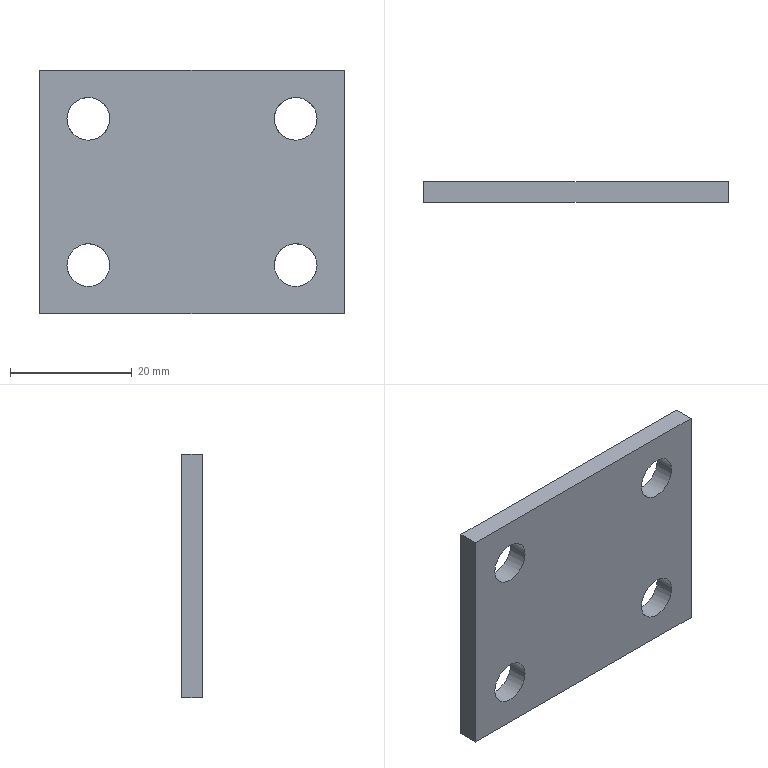Part | STEP file | Positioning_id2146_x_t | 1 solid | 14 faces | box 50 x 3.35 x 40 mm | volume 6184 mm3 | cylinder 8 | plane 6 | commonest cylinder face diameters 7 x8
STEP:
#1=CARTESIAN_POINT('',(0.,0.,0.));
#2=DIRECTION('',(0.,0.,1.));
#3=DIRECTION('',(1.,0.,0.));
#4=AXIS2_PLACEMENT_3D('',#1,#2,#3);
#5=CARTESIAN_POINT('',(-816.502,-53.35,344.5));
#6=VERTEX_POINT('',#5);
#7=CARTESIAN_POINT('',(-823.502,-53.35,344.5));
#8=VERTEX_POINT('',#7);
#9=CARTESIAN_POINT('',(-820.002,-53.35,344.5));
#10=DIRECTION('',(0.,-1.,0.));
#11=DIRECTION('',(1.,0.,0.));
#12=AXIS2_PLACEMENT_3D('',#9,#10,#11);
#13=CIRCLE('',#12,3.5);
#14=CARTESIAN_POINT('',(-773.002,-53.35,376.5));
#15=DIRECTION('',(0.,1.,0.));
#16=DIRECTION('',(-1.,0.,0.));
#17=AXIS2_PLACEMENT_3D('',#14,#15,#16);
#18=PLANE('',#17);
#19=CARTESIAN_POINT('',(43.5,-32.));
#20=CARTESIAN_POINT('',(43.5,-25.938));
#21=CARTESIAN_POINT('',(48.75,-28.969));
#22=CARTESIAN_POINT('',(54.,-32.));
#23=CARTESIAN_POINT('',(48.75,-35.031));
#24=CARTESIAN_POINT('',(43.5,-38.062));
#25=CARTESIAN_POINT('',(43.5,-32.));
#26=(BOUNDED_CURVE()B_SPLINE_CURVE(2,(#19,#20,#21,#22,#23,#24,#25),.UNSPECIFIED.,.T.,.F.)B_SPLINE_CURVE_WITH_KNOTS((1,2,2,2,2,1),(-2.094,0.,2.094,4.189,6.283,8.378),.UNSPECIFIED.)CURVE()GEOMETRIC_REPRESENTATION_ITEM()RATIONAL_B_SPLINE_CURVE((1.,0.5,1.,0.5,1.,0.5,1.))REPRESENTATION_ITEM(''));
#27=(GEOMETRIC_REPRESENTATION_CONTEXT(2)PARAMETRIC_REPRESENTATION_CONTEXT()REPRESENTATION_CONTEXT('',''));
#28=DEFINITIONAL_REPRESENTATION('',(#26),#27);
#29=PCURVE('',#18,#28);
#30=CARTESIAN_POINT('',(-820.002,-66.,344.5));
#31=DIRECTION('',(0.,-1.,0.));
#32=DIRECTION('',(-1.,0.,0.));
#33=AXIS2_PLACEMENT_3D('',#30,#31,#32);
#34=CYLINDRICAL_SURFACE('',#33,3.5);
#35=CARTESIAN_POINT('',(3.142,-12.65));
#36=DIRECTION('',(1.,0.));
#37=VECTOR('',#36,1.);
#38=LINE('',#35,#37);
#39=(GEOMETRIC_REPRESENTATION_CONTEXT(2)PARAMETRIC_REPRESENTATION_CONTEXT()REPRESENTATION_CONTEXT('',''));
#40=DEFINITIONAL_REPRESENTATION('',(#38),#39);
#41=PCURVE('',#34,#40);
#42=SURFACE_CURVE('',#13,(#29,#41),.PCURVE_S1.);
#43=EDGE_CURVE('',#6,#8,#42,.T.);
#44=ORIENTED_EDGE('',*,*,#43,.F.);
#45=CARTESIAN_POINT('',(-820.002,-53.35,341.));
#46=VERTEX_POINT('',#45);
#47=CARTESIAN_POINT('',(-820.002,-53.35,344.5));
#48=DIRECTION('',(0.,-1.,0.));
#49=DIRECTION('',(0.,0.,-1.));
#50=AXIS2_PLACEMENT_3D('',#47,#48,#49);
#51=CIRCLE('',#50,3.5);
#52=CARTESIAN_POINT('',(47.,-35.5));
#53=CARTESIAN_POINT('',(40.938,-35.5));
#54=CARTESIAN_POINT('',(43.969,-30.25));
#55=CARTESIAN_POINT('',(47.,-25.));
#56=CARTESIAN_POINT('',(50.031,-30.25));
#57=CARTESIAN_POINT('',(53.062,-35.5));
#58=CARTESIAN_POINT('',(47.,-35.5));
#59=(BOUNDED_CURVE()B_SPLINE_CURVE(2,(#52,#53,#54,#55,#56,#57,#58),.UNSPECIFIED.,.T.,.F.)B_SPLINE_CURVE_WITH_KNOTS((1,2,2,2,2,1),(-2.094,0.,2.094,4.189,6.283,8.378),.UNSPECIFIED.)CURVE()GEOMETRIC_REPRESENTATION_ITEM()RATIONAL_B_SPLINE_CURVE((1.,0.5,1.,0.5,1.,0.5,1.))REPRESENTATION_ITEM(''));
#60=(GEOMETRIC_REPRESENTATION_CONTEXT(2)PARAMETRIC_REPRESENTATION_CONTEXT()REPRESENTATION_CONTEXT('',''));
#61=DEFINITIONAL_REPRESENTATION('',(#59),#60);
#62=PCURVE('',#18,#61);
#63=CARTESIAN_POINT('',(-820.002,-66.,344.5));
#64=DIRECTION('',(0.,-1.,0.));
#65=DIRECTION('',(-1.,0.,0.));
#66=AXIS2_PLACEMENT_3D('',#63,#64,#65);
#67=CYLINDRICAL_SURFACE('',#66,3.5);
#68=CARTESIAN_POINT('',(1.571,-12.65));
#69=DIRECTION('',(1.,0.));
#70=VECTOR('',#69,1.);
#71=LINE('',#68,#70);
#72=(GEOMETRIC_REPRESENTATION_CONTEXT(2)PARAMETRIC_REPRESENTATION_CONTEXT()REPRESENTATION_CONTEXT('',''));
#73=DEFINITIONAL_REPRESENTATION('',(#71),#72);
#74=PCURVE('',#67,#73);
#75=SURFACE_CURVE('',#51,(#62,#74),.PCURVE_S1.);
#76=EDGE_CURVE('',#46,#6,#75,.T.);
#77=ORIENTED_EDGE('',*,*,#76,.F.);
#78=CARTESIAN_POINT('',(-820.002,-53.35,344.5));
#79=DIRECTION('',(0.,-1.,0.));
#80=DIRECTION('',(-1.,0.,0.));
#81=AXIS2_PLACEMENT_3D('',#78,#79,#80);
#82=CIRCLE('',#81,3.5);
#83=CARTESIAN_POINT('',(50.5,-32.));
#84=CARTESIAN_POINT('',(50.5,-38.062));
#85=CARTESIAN_POINT('',(45.25,-35.031));
#86=CARTESIAN_POINT('',(40.,-32.));
#87=CARTESIAN_POINT('',(45.25,-28.969));
#88=CARTESIAN_POINT('',(50.5,-25.938));
#89=CARTESIAN_POINT('',(50.5,-32.));
#90=(BOUNDED_CURVE()B_SPLINE_CURVE(2,(#83,#84,#85,#86,#87,#88,#89),.UNSPECIFIED.,.T.,.F.)B_SPLINE_CURVE_WITH_KNOTS((1,2,2,2,2,1),(-2.094,0.,2.094,4.189,6.283,8.378),.UNSPECIFIED.)CURVE()GEOMETRIC_REPRESENTATION_ITEM()RATIONAL_B_SPLINE_CURVE((1.,0.5,1.,0.5,1.,0.5,1.))REPRESENTATION_ITEM(''));
#91=(GEOMETRIC_REPRESENTATION_CONTEXT(2)PARAMETRIC_REPRESENTATION_CONTEXT()REPRESENTATION_CONTEXT('',''));
#92=DEFINITIONAL_REPRESENTATION('',(#90),#91);
#93=PCURVE('',#18,#92);
#94=CARTESIAN_POINT('',(0.,-12.65));
#95=DIRECTION('',(1.,0.));
#96=VECTOR('',#95,1.);
#97=LINE('',#94,#96);
#98=(GEOMETRIC_REPRESENTATION_CONTEXT(2)PARAMETRIC_REPRESENTATION_CONTEXT()REPRESENTATION_CONTEXT('',''));
#99=DEFINITIONAL_REPRESENTATION('',(#97),#98);
#100=PCURVE('',#67,#99);
#101=SURFACE_CURVE('',#82,(#93,#100),.PCURVE_S1.);
#102=EDGE_CURVE('',#8,#46,#101,.T.);
#103=ORIENTED_EDGE('',*,*,#102,.F.);
#104=EDGE_LOOP('',(#44,#77,#103));
#105=FACE_BOUND('',#104,.T.);
#106=CARTESIAN_POINT('',(-782.502,-53.35,368.5));
#107=VERTEX_POINT('',#106);
#108=CARTESIAN_POINT('',(-789.502,-53.35,368.5));
#109=VERTEX_POINT('',#108);
#110=CARTESIAN_POINT('',(-786.002,-53.35,368.5));
#111=DIRECTION('',(0.,-1.,0.));
#112=DIRECTION('',(1.,0.,0.));
#113=AXIS2_PLACEMENT_3D('',#110,#111,#112);
#114=CIRCLE('',#113,3.5);
#115=CARTESIAN_POINT('',(9.5,-8.));
#116=CARTESIAN_POINT('',(9.5,-1.938));
#117=CARTESIAN_POINT('',(14.75,-4.969));
#118=CARTESIAN_POINT('',(20.,-8.));
#119=CARTESIAN_POINT('',(14.75,-11.031));
#120=CARTESIAN_POINT('',(9.5,-14.062));
#121=CARTESIAN_POINT('',(9.5,-8.));
#122=(BOUNDED_CURVE()B_SPLINE_CURVE(2,(#115,#116,#117,#118,#119,#120,#121),.UNSPECIFIED.,.T.,.F.)B_SPLINE_CURVE_WITH_KNOTS((1,2,2,2,2,1),(-2.094,0.,2.094,4.189,6.283,8.378),.UNSPECIFIED.)CURVE()GEOMETRIC_REPRESENTATION_ITEM()RATIONAL_B_SPLINE_CURVE((1.,0.5,1.,0.5,1.,0.5,1.))REPRESENTATION_ITEM(''));
#123=(GEOMETRIC_REPRESENTATION_CONTEXT(2)PARAMETRIC_REPRESENTATION_CONTEXT()REPRESENTATION_CONTEXT('',''));
#124=DEFINITIONAL_REPRESENTATION('',(#122),#123);
#125=PCURVE('',#18,#124);
#126=CARTESIAN_POINT('',(-786.002,-66.,368.5));
#127=DIRECTION('',(0.,-1.,0.));
#128=DIRECTION('',(-1.,0.,0.));
#129=AXIS2_PLACEMENT_3D('',#126,#127,#128);
#130=CYLINDRICAL_SURFACE('',#129,3.5);
#131=CARTESIAN_POINT('',(3.142,-12.65));
#132=DIRECTION('',(1.,0.));
#133=VECTOR('',#132,1.);
#134=LINE('',#131,#133);
#135=(GEOMETRIC_REPRESENTATION_CONTEXT(2)PARAMETRIC_REPRESENTATION_CONTEXT()REPRESENTATION_CONTEXT('',''));
#136=DEFINITIONAL_REPRESENTATION('',(#134),#135);
#137=PCURVE('',#130,#136);
#138=SURFACE_CURVE('',#114,(#125,#137),.PCURVE_S1.);
#139=EDGE_CURVE('',#107,#109,#138,.T.);
#140=ORIENTED_EDGE('',*,*,#139,.F.);
#141=CARTESIAN_POINT('',(-786.002,-53.35,365.));
#142=VERTEX_POINT('',#141);
#143=CARTESIAN_POINT('',(-786.002,-53.35,368.5));
#144=DIRECTION('',(0.,-1.,0.));
#145=DIRECTION('',(0.,0.,-1.));
#146=AXIS2_PLACEMENT_3D('',#143,#144,#145);
#147=CIRCLE('',#146,3.5);
#148=CARTESIAN_POINT('',(13.,-11.5));
#149=CARTESIAN_POINT('',(6.938,-11.5));
#150=CARTESIAN_POINT('',(9.969,-6.25));
#151=CARTESIAN_POINT('',(13.,-1.));
#152=CARTESIAN_POINT('',(16.031,-6.25));
#153=CARTESIAN_POINT('',(19.062,-11.5));
#154=CARTESIAN_POINT('',(13.,-11.5));
#155=(BOUNDED_CURVE()B_SPLINE_CURVE(2,(#148,#149,#150,#151,#152,#153,#154),.UNSPECIFIED.,.T.,.F.)B_SPLINE_CURVE_WITH_KNOTS((1,2,2,2,2,1),(-2.094,0.,2.094,4.189,6.283,8.378),.UNSPECIFIED.)CURVE()GEOMETRIC_REPRESENTATION_ITEM()RATIONAL_B_SPLINE_CURVE((1.,0.5,1.,0.5,1.,0.5,1.))REPRESENTATION_ITEM(''));
#156=(GEOMETRIC_REPRESENTATION_CONTEXT(2)PARAMETRIC_REPRESENTATION_CONTEXT()REPRESENTATION_CONTEXT('',''));
#157=DEFINITIONAL_REPRESENTATION('',(#155),#156);
#158=PCURVE('',#18,#157);
#159=CARTESIAN_POINT('',(-786.002,-66.,368.5));
#160=DIRECTION('',(0.,-1.,0.));
#161=DIRECTION('',(-1.,0.,0.));
#162=AXIS2_PLACEMENT_3D('',#159,#160,#161);
#163=CYLINDRICAL_SURFACE('',#162,3.5);
#164=CARTESIAN_POINT('',(1.571,-12.65));
#165=DIRECTION('',(1.,0.));
#166=VECTOR('',#165,1.);
#167=LINE('',#164,#166);
#168=(GEOMETRIC_REPRESENTATION_CONTEXT(2)PARAMETRIC_REPRESENTATION_CONTEXT()REPRESENTATION_CONTEXT('',''));
#169=DEFINITIONAL_REPRESENTATION('',(#167),#168);
#170=PCURVE('',#163,#169);
#171=SURFACE_CURVE('',#147,(#158,#170),.PCURVE_S1.);
#172=EDGE_CURVE('',#142,#107,#171,.T.);
#173=ORIENTED_EDGE('',*,*,#172,.F.);
#174=CARTESIAN_POINT('',(-786.002,-53.35,368.5));
#175=DIRECTION('',(0.,-1.,0.));
#176=DIRECTION('',(-1.,0.,0.));
#177=AXIS2_PLACEMENT_3D('',#174,#175,#176);
#178=CIRCLE('',#177,3.5);
#179=CARTESIAN_POINT('',(16.5,-8.));
#180=CARTESIAN_POINT('',(16.5,-14.062));
#181=CARTESIAN_POINT('',(11.25,-11.031));
#182=CARTESIAN_POINT('',(6.,-8.));
#183=CARTESIAN_POINT('',(11.25,-4.969));
#184=CARTESIAN_POINT('',(16.5,-1.938));
#185=CARTESIAN_POINT('',(16.5,-8.));
#186=(BOUNDED_CURVE()B_SPLINE_CURVE(2,(#179,#180,#181,#182,#183,#184,#185),.UNSPECIFIED.,.T.,.F.)B_SPLINE_CURVE_WITH_KNOTS((1,2,2,2,2,1),(-2.094,0.,2.094,4.189,6.283,8.378),.UNSPECIFIED.)CURVE()GEOMETRIC_REPRESENTATION_ITEM()RATIONAL_B_SPLINE_CURVE((1.,0.5,1.,0.5,1.,0.5,1.))REPRESENTATION_ITEM(''));
#187=(GEOMETRIC_REPRESENTATION_CONTEXT(2)PARAMETRIC_REPRESENTATION_CONTEXT()REPRESENTATION_CONTEXT('',''));
#188=DEFINITIONAL_REPRESENTATION('',(#186),#187);
#189=PCURVE('',#18,#188);
#190=CARTESIAN_POINT('',(0.,-12.65));
#191=DIRECTION('',(1.,0.));
#192=VECTOR('',#191,1.);
#193=LINE('',#190,#192);
#194=(GEOMETRIC_REPRESENTATION_CONTEXT(2)PARAMETRIC_REPRESENTATION_CONTEXT()REPRESENTATION_CONTEXT('',''));
#195=DEFINITIONAL_REPRESENTATION('',(#193),#194);
#196=PCURVE('',#163,#195);
#197=SURFACE_CURVE('',#178,(#189,#196),.PCURVE_S1.);
#198=EDGE_CURVE('',#109,#142,#197,.T.);
#199=ORIENTED_EDGE('',*,*,#198,.F.);
#200=EDGE_LOOP('',(#140,#173,#199));
#201=FACE_BOUND('',#200,.T.);
#202=CARTESIAN_POINT('',(-782.502,-53.35,344.5));
#203=VERTEX_POINT('',#202);
#204=CARTESIAN_POINT('',(-789.502,-53.35,344.5));
#205=VERTEX_POINT('',#204);
#206=CARTESIAN_POINT('',(-786.002,-53.35,344.5));
#207=DIRECTION('',(0.,-1.,0.));
#208=DIRECTION('',(1.,0.,0.));
#209=AXIS2_PLACEMENT_3D('',#206,#207,#208);
#210=CIRCLE('',#209,3.5);
#211=CARTESIAN_POINT('',(9.5,-32.));
#212=CARTESIAN_POINT('',(9.5,-25.938));
#213=CARTESIAN_POINT('',(14.75,-28.969));
#214=CARTESIAN_POINT('',(20.,-32.));
#215=CARTESIAN_POINT('',(14.75,-35.031));
#216=CARTESIAN_POINT('',(9.5,-38.062));
#217=CARTESIAN_POINT('',(9.5,-32.));
#218=(BOUNDED_CURVE()B_SPLINE_CURVE(2,(#211,#212,#213,#214,#215,#216,#217),.UNSPECIFIED.,.T.,.F.)B_SPLINE_CURVE_WITH_KNOTS((1,2,2,2,2,1),(-2.094,0.,2.094,4.189,6.283,8.378),.UNSPECIFIED.)CURVE()GEOMETRIC_REPRESENTATION_ITEM()RATIONAL_B_SPLINE_CURVE((1.,0.5,1.,0.5,1.,0.5,1.))REPRESENTATION_ITEM(''));
#219=(GEOMETRIC_REPRESENTATION_CONTEXT(2)PARAMETRIC_REPRESENTATION_CONTEXT()REPRESENTATION_CONTEXT('',''));
#220=DEFINITIONAL_REPRESENTATION('',(#218),#219);
#221=PCURVE('',#18,#220);
#222=CARTESIAN_POINT('',(-786.002,-66.,344.5));
#223=DIRECTION('',(0.,-1.,0.));
#224=DIRECTION('',(-1.,0.,0.));
#225=AXIS2_PLACEMENT_3D('',#222,#223,#224);
#226=CYLINDRICAL_SURFACE('',#225,3.5);
#227=CARTESIAN_POINT('',(3.142,-12.65));
#228=DIRECTION('',(1.,0.));
#229=VECTOR('',#228,1.);
#230=LINE('',#227,#229);
#231=(GEOMETRIC_REPRESENTATION_CONTEXT(2)PARAMETRIC_REPRESENTATION_CONTEXT()REPRESENTATION_CONTEXT('',''));
#232=DEFINITIONAL_REPRESENTATION('',(#230),#231);
#233=PCURVE('',#226,#232);
#234=SURFACE_CURVE('',#210,(#221,#233),.PCURVE_S1.);
#235=EDGE_CURVE('',#203,#205,#234,.T.);
#236=ORIENTED_EDGE('',*,*,#235,.F.);
#237=CARTESIAN_POINT('',(-786.002,-53.35,341.));
#238=VERTEX_POINT('',#237);
#239=CARTESIAN_POINT('',(-786.002,-53.35,344.5));
#240=DIRECTION('',(0.,-1.,0.));
#241=DIRECTION('',(0.,0.,-1.));
#242=AXIS2_PLACEMENT_3D('',#239,#240,#241);
#243=CIRCLE('',#242,3.5);
#244=CARTESIAN_POINT('',(13.,-35.5));
#245=CARTESIAN_POINT('',(6.938,-35.5));
#246=CARTESIAN_POINT('',(9.969,-30.25));
#247=CARTESIAN_POINT('',(13.,-25.));
#248=CARTESIAN_POINT('',(16.031,-30.25));
#249=CARTESIAN_POINT('',(19.062,-35.5));
#250=CARTESIAN_POINT('',(13.,-35.5));
#251=(BOUNDED_CURVE()B_SPLINE_CURVE(2,(#244,#245,#246,#247,#248,#249,#250),.UNSPECIFIED.,.T.,.F.)B_SPLINE_CURVE_WITH_KNOTS((1,2,2,2,2,1),(-2.094,0.,2.094,4.189,6.283,8.378),.UNSPECIFIED.)CURVE()GEOMETRIC_REPRESENTATION_ITEM()RATIONAL_B_SPLINE_CURVE((1.,0.5,1.,0.5,1.,0.5,1.))REPRESENTATION_ITEM(''));
#252=(GEOMETRIC_REPRESENTATION_CONTEXT(2)PARAMETRIC_REPRESENTATION_CONTEXT()REPRESENTATION_CONTEXT('',''));
#253=DEFINITIONAL_REPRESENTATION('',(#251),#252);
#254=PCURVE('',#18,#253);
#255=CARTESIAN_POINT('',(-786.002,-66.,344.5));
#256=DIRECTION('',(0.,-1.,0.));
#257=DIRECTION('',(-1.,0.,0.));
#258=AXIS2_PLACEMENT_3D('',#255,#256,#257);
#259=CYLINDRICAL_SURFACE('',#258,3.5);
#260=CARTESIAN_POINT('',(1.571,-12.65));
#261=DIRECTION('',(1.,0.));
#262=VECTOR('',#261,1.);
#263=LINE('',#260,#262);
#264=(GEOMETRIC_REPRESENTATION_CONTEXT(2)PARAMETRIC_REPRESENTATION_CONTEXT()REPRESENTATION_CONTEXT('',''));
#265=DEFINITIONAL_REPRESENTATION('',(#263),#264);
#266=PCURVE('',#259,#265);
#267=SURFACE_CURVE('',#243,(#254,#266),.PCURVE_S1.);
#268=EDGE_CURVE('',#238,#203,#267,.T.);
#269=ORIENTED_EDGE('',*,*,#268,.F.);
#270=CARTESIAN_POINT('',(-786.002,-53.35,344.5));
#271=DIRECTION('',(0.,-1.,0.));
#272=DIRECTION('',(-1.,0.,0.));
#273=AXIS2_PLACEMENT_3D('',#270,#271,#272);
#274=CIRCLE('',#273,3.5);
#275=CARTESIAN_POINT('',(16.5,-32.));
#276=CARTESIAN_POINT('',(16.5,-38.062));
#277=CARTESIAN_POINT('',(11.25,-35.031));
#278=CARTESIAN_POINT('',(6.,-32.));
#279=CARTESIAN_POINT('',(11.25,-28.969));
#280=CARTESIAN_POINT('',(16.5,-25.938));
#281=CARTESIAN_POINT('',(16.5,-32.));
#282=(BOUNDED_CURVE()B_SPLINE_CURVE(2,(#275,#276,#277,#278,#279,#280,#281),.UNSPECIFIED.,.T.,.F.)B_SPLINE_CURVE_WITH_KNOTS((1,2,2,2,2,1),(-2.094,0.,2.094,4.189,6.283,8.378),.UNSPECIFIED.)CURVE()GEOMETRIC_REPRESENTATION_ITEM()RATIONAL_B_SPLINE_CURVE((1.,0.5,1.,0.5,1.,0.5,1.))REPRESENTATION_ITEM(''));
#283=(GEOMETRIC_REPRESENTATION_CONTEXT(2)PARAMETRIC_REPRESENTATION_CONTEXT()REPRESENTATION_CONTEXT('',''));
#284=DEFINITIONAL_REPRESENTATION('',(#282),#283);
#285=PCURVE('',#18,#284);
#286=CARTESIAN_POINT('',(0.,-12.65));
#287=DIRECTION('',(1.,0.));
#288=VECTOR('',#287,1.);
#289=LINE('',#286,#288);
#290=(GEOMETRIC_REPRESENTATION_CONTEXT(2)PARAMETRIC_REPRESENTATION_CONTEXT()REPRESENTATION_CONTEXT('',''));
#291=DEFINITIONAL_REPRESENTATION('',(#289),#290);
#292=PCURVE('',#259,#291);
#293=SURFACE_CURVE('',#274,(#285,#292),.PCURVE_S1.);
#294=EDGE_CURVE('',#205,#238,#293,.T.);
#295=ORIENTED_EDGE('',*,*,#294,.F.);
#296=EDGE_LOOP('',(#236,#269,#295));
#297=FACE_BOUND('',#296,.T.);
#298=CARTESIAN_POINT('',(-816.502,-53.35,368.5));
#299=VERTEX_POINT('',#298);
#300=CARTESIAN_POINT('',(-823.502,-53.35,368.5));
#301=VERTEX_POINT('',#300);
#302=CARTESIAN_POINT('',(-820.002,-53.35,368.5));
#303=DIRECTION('',(0.,-1.,0.));
#304=DIRECTION('',(1.,0.,0.));
#305=AXIS2_PLACEMENT_3D('',#302,#303,#304);
#306=CIRCLE('',#305,3.5);
#307=CARTESIAN_POINT('',(43.5,-8.));
#308=CARTESIAN_POINT('',(43.5,-1.938));
#309=CARTESIAN_POINT('',(48.75,-4.969));
#310=CARTESIAN_POINT('',(54.,-8.));
#311=CARTESIAN_POINT('',(48.75,-11.031));
#312=CARTESIAN_POINT('',(43.5,-14.062));
#313=CARTESIAN_POINT('',(43.5,-8.));
#314=(BOUNDED_CURVE()B_SPLINE_CURVE(2,(#307,#308,#309,#310,#311,#312,#313),.UNSPECIFIED.,.T.,.F.)B_SPLINE_CURVE_WITH_KNOTS((1,2,2,2,2,1),(-2.094,0.,2.094,4.189,6.283,8.378),.UNSPECIFIED.)CURVE()GEOMETRIC_REPRESENTATION_ITEM()RATIONAL_B_SPLINE_CURVE((1.,0.5,1.,0.5,1.,0.5,1.))REPRESENTATION_ITEM(''));
#315=(GEOMETRIC_REPRESENTATION_CONTEXT(2)PARAMETRIC_REPRESENTATION_CONTEXT()REPRESENTATION_CONTEXT('',''));
#316=DEFINITIONAL_REPRESENTATION('',(#314),#315);
#317=PCURVE('',#18,#316);
#318=CARTESIAN_POINT('',(-820.002,-66.,368.5));
#319=DIRECTION('',(0.,-1.,0.));
#320=DIRECTION('',(-1.,0.,0.));
#321=AXIS2_PLACEMENT_3D('',#318,#319,#320);
#322=CYLINDRICAL_SURFACE('',#321,3.5);
#323=CARTESIAN_POINT('',(3.142,-12.65));
#324=DIRECTION('',(1.,0.));
#325=VECTOR('',#324,1.);
#326=LINE('',#323,#325);
#327=(GEOMETRIC_REPRESENTATION_CONTEXT(2)PARAMETRIC_REPRESENTATION_CONTEXT()REPRESENTATION_CONTEXT('',''));
#328=DEFINITIONAL_REPRESENTATION('',(#326),#327);
#329=PCURVE('',#322,#328);
#330=SURFACE_CURVE('',#306,(#317,#329),.PCURVE_S1.);
#331=EDGE_CURVE('',#299,#301,#330,.T.);
#332=ORIENTED_EDGE('',*,*,#331,.F.);
#333=CARTESIAN_POINT('',(-820.002,-53.35,365.));
#334=VERTEX_POINT('',#333);
#335=CARTESIAN_POINT('',(-820.002,-53.35,368.5));
#336=DIRECTION('',(0.,-1.,0.));
#337=DIRECTION('',(0.,0.,-1.));
#338=AXIS2_PLACEMENT_3D('',#335,#336,#337);
#339=CIRCLE('',#338,3.5);
#340=CARTESIAN_POINT('',(47.,-11.5));
#341=CARTESIAN_POINT('',(40.938,-11.5));
#342=CARTESIAN_POINT('',(43.969,-6.25));
#343=CARTESIAN_POINT('',(47.,-1.));
#344=CARTESIAN_POINT('',(50.031,-6.25));
#345=CARTESIAN_POINT('',(53.062,-11.5));
#346=CARTESIAN_POINT('',(47.,-11.5));
#347=(BOUNDED_CURVE()B_SPLINE_CURVE(2,(#340,#341,#342,#343,#344,#345,#346),.UNSPECIFIED.,.T.,.F.)B_SPLINE_CURVE_WITH_KNOTS((1,2,2,2,2,1),(-2.094,0.,2.094,4.189,6.283,8.378),.UNSPECIFIED.)CURVE()GEOMETRIC_REPRESENTATION_ITEM()RATIONAL_B_SPLINE_CURVE((1.,0.5,1.,0.5,1.,0.5,1.))REPRESENTATION_ITEM(''));
#348=(GEOMETRIC_REPRESENTATION_CONTEXT(2)PARAMETRIC_REPRESENTATION_CONTEXT()REPRESENTATION_CONTEXT('',''));
#349=DEFINITIONAL_REPRESENTATION('',(#347),#348);
#350=PCURVE('',#18,#349);
#351=CARTESIAN_POINT('',(-820.002,-66.,368.5));
#352=DIRECTION('',(0.,-1.,0.));
#353=DIRECTION('',(-1.,0.,0.));
#354=AXIS2_PLACEMENT_3D('',#351,#352,#353);
#355=CYLINDRICAL_SURFACE('',#354,3.5);
#356=CARTESIAN_POINT('',(1.571,-12.65));
#357=DIRECTION('',(1.,0.));
#358=VECTOR('',#357,1.);
#359=LINE('',#356,#358);
#360=(GEOMETRIC_REPRESENTATION_CONTEXT(2)PARAMETRIC_REPRESENTATION_CONTEXT()REPRESENTATION_CONTEXT('',''));
#361=DEFINITIONAL_REPRESENTATION('',(#359),#360);
#362=PCURVE('',#355,#361);
#363=SURFACE_CURVE('',#339,(#350,#362),.PCURVE_S1.);
#364=EDGE_CURVE('',#334,#299,#363,.T.);
#365=ORIENTED_EDGE('',*,*,#364,.F.);
#366=CARTESIAN_POINT('',(-820.002,-53.35,368.5));
#367=DIRECTION('',(0.,-1.,0.));
#368=DIRECTION('',(-1.,0.,0.));
#369=AXIS2_PLACEMENT_3D('',#366,#367,#368);
#370=CIRCLE('',#369,3.5);
#371=CARTESIAN_POINT('',(50.5,-8.));
#372=CARTESIAN_POINT('',(50.5,-14.062));
#373=CARTESIAN_POINT('',(45.25,-11.031));
#374=CARTESIAN_POINT('',(40.,-8.));
#375=CARTESIAN_POINT('',(45.25,-4.969));
#376=CARTESIAN_POINT('',(50.5,-1.938));
#377=CARTESIAN_POINT('',(50.5,-8.));
#378=(BOUNDED_CURVE()B_SPLINE_CURVE(2,(#371,#372,#373,#374,#375,#376,#377),.UNSPECIFIED.,.T.,.F.)B_SPLINE_CURVE_WITH_KNOTS((1,2,2,2,2,1),(-2.094,0.,2.094,4.189,6.283,8.378),.UNSPECIFIED.)CURVE()GEOMETRIC_REPRESENTATION_ITEM()RATIONAL_B_SPLINE_CURVE((1.,0.5,1.,0.5,1.,0.5,1.))REPRESENTATION_ITEM(''));
#379=(GEOMETRIC_REPRESENTATION_CONTEXT(2)PARAMETRIC_REPRESENTATION_CONTEXT()REPRESENTATION_CONTEXT('',''));
#380=DEFINITIONAL_REPRESENTATION('',(#378),#379);
#381=PCURVE('',#18,#380);
#382=CARTESIAN_POINT('',(0.,-12.65));
#383=DIRECTION('',(1.,0.));
#384=VECTOR('',#383,1.);
#385=LINE('',#382,#384);
#386=(GEOMETRIC_REPRESENTATION_CONTEXT(2)PARAMETRIC_REPRESENTATION_CONTEXT()REPRESENTATION_CONTEXT('',''));
#387=DEFINITIONAL_REPRESENTATION('',(#385),#386);
#388=PCURVE('',#355,#387);
#389=SURFACE_CURVE('',#370,(#381,#388),.PCURVE_S1.);
#390=EDGE_CURVE('',#301,#334,#389,.T.);
#391=ORIENTED_EDGE('',*,*,#390,.F.);
#392=EDGE_LOOP('',(#332,#365,#391));
#393=FACE_BOUND('',#392,.T.);
#394=CARTESIAN_POINT('',(-828.002,-53.35,336.5));
#395=VERTEX_POINT('',#394);
#396=CARTESIAN_POINT('',(-778.002,-53.35,336.5));
#397=VERTEX_POINT('',#396);
#398=CARTESIAN_POINT('',(-828.002,-53.35,336.5));
#399=DIRECTION('',(1.,0.,0.));
#400=VECTOR('',#399,1.);
#401=LINE('',#398,#400);
#402=CARTESIAN_POINT('',(55.,-40.));
#403=DIRECTION('',(-1.,0.));
#404=VECTOR('',#403,1.);
#405=LINE('',#402,#404);
#406=(GEOMETRIC_REPRESENTATION_CONTEXT(2)PARAMETRIC_REPRESENTATION_CONTEXT()REPRESENTATION_CONTEXT('',''));
#407=DEFINITIONAL_REPRESENTATION('',(#405),#406);
#408=PCURVE('',#18,#407);
#409=CARTESIAN_POINT('',(-826.775,-17.,336.5));
#410=DIRECTION('',(0.,0.,-1.));
#411=DIRECTION('',(0.,-1.,0.));
#412=AXIS2_PLACEMENT_3D('',#409,#410,#411);
#413=PLANE('',#412);
#414=CARTESIAN_POINT('',(36.35,1.227));
#415=DIRECTION('',(0.,-1.));
#416=VECTOR('',#415,1.);
#417=LINE('',#414,#416);
#418=(GEOMETRIC_REPRESENTATION_CONTEXT(2)PARAMETRIC_REPRESENTATION_CONTEXT()REPRESENTATION_CONTEXT('',''));
#419=DEFINITIONAL_REPRESENTATION('',(#417),#418);
#420=PCURVE('',#413,#419);
#421=SURFACE_CURVE('',#401,(#408,#420),.PCURVE_S1.);
#422=EDGE_CURVE('',#395,#397,#421,.T.);
#423=ORIENTED_EDGE('',*,*,#422,.T.);
#424=CARTESIAN_POINT('',(-778.002,-53.35,376.5));
#425=VERTEX_POINT('',#424);
#426=CARTESIAN_POINT('',(-778.002,-53.35,336.5));
#427=DIRECTION('',(0.,0.,1.));
#428=VECTOR('',#427,1.);
#429=LINE('',#426,#428);
#430=CARTESIAN_POINT('',(5.,-40.));
#431=DIRECTION('',(0.,1.));
#432=VECTOR('',#431,1.);
#433=LINE('',#430,#432);
#434=(GEOMETRIC_REPRESENTATION_CONTEXT(2)PARAMETRIC_REPRESENTATION_CONTEXT()REPRESENTATION_CONTEXT('',''));
#435=DEFINITIONAL_REPRESENTATION('',(#433),#434);
#436=PCURVE('',#18,#435);
#437=CARTESIAN_POINT('',(-778.002,-46.,376.5));
#438=DIRECTION('',(1.,0.,0.));
#439=DIRECTION('',(0.,1.,0.));
#440=AXIS2_PLACEMENT_3D('',#437,#438,#439);
#441=PLANE('',#440);
#442=CARTESIAN_POINT('',(-7.35,-40.));
#443=DIRECTION('',(0.,1.));
#444=VECTOR('',#443,1.);
#445=LINE('',#442,#444);
#446=(GEOMETRIC_REPRESENTATION_CONTEXT(2)PARAMETRIC_REPRESENTATION_CONTEXT()REPRESENTATION_CONTEXT('',''));
#447=DEFINITIONAL_REPRESENTATION('',(#445),#446);
#448=PCURVE('',#441,#447);
#449=SURFACE_CURVE('',#429,(#436,#448),.PCURVE_S1.);
#450=EDGE_CURVE('',#397,#425,#449,.T.);
#451=ORIENTED_EDGE('',*,*,#450,.T.);
#452=CARTESIAN_POINT('',(-828.002,-53.35,376.5));
#453=VERTEX_POINT('',#452);
#454=CARTESIAN_POINT('',(-778.002,-53.35,376.5));
#455=DIRECTION('',(-1.,0.,0.));
#456=VECTOR('',#455,1.);
#457=LINE('',#454,#456);
#458=CARTESIAN_POINT('',(5.,0.));
#459=DIRECTION('',(1.,0.));
#460=VECTOR('',#459,1.);
#461=LINE('',#458,#460);
#462=(GEOMETRIC_REPRESENTATION_CONTEXT(2)PARAMETRIC_REPRESENTATION_CONTEXT()REPRESENTATION_CONTEXT('',''));
#463=DEFINITIONAL_REPRESENTATION('',(#461),#462);
#464=PCURVE('',#18,#463);
#465=CARTESIAN_POINT('',(-826.775,-17.,376.5));
#466=DIRECTION('',(0.,0.,1.));
#467=DIRECTION('',(0.,1.,0.));
#468=AXIS2_PLACEMENT_3D('',#465,#466,#467);
#469=PLANE('',#468);
#470=CARTESIAN_POINT('',(-36.35,-48.773));
#471=DIRECTION('',(0.,1.));
#472=VECTOR('',#471,1.);
#473=LINE('',#470,#472);
#474=(GEOMETRIC_REPRESENTATION_CONTEXT(2)PARAMETRIC_REPRESENTATION_CONTEXT()REPRESENTATION_CONTEXT('',''));
#475=DEFINITIONAL_REPRESENTATION('',(#473),#474);
#476=PCURVE('',#469,#475);
#477=SURFACE_CURVE('',#457,(#464,#476),.PCURVE_S1.);
#478=EDGE_CURVE('',#425,#453,#477,.T.);
#479=ORIENTED_EDGE('',*,*,#478,.T.);
#480=CARTESIAN_POINT('',(-828.002,-53.35,336.5));
#481=DIRECTION('',(0.,0.,1.));
#482=VECTOR('',#481,1.);
#483=LINE('',#480,#482);
#484=CARTESIAN_POINT('',(55.,-40.));
#485=DIRECTION('',(0.,1.));
#486=VECTOR('',#485,1.);
#487=LINE('',#484,#486);
#488=(GEOMETRIC_REPRESENTATION_CONTEXT(2)PARAMETRIC_REPRESENTATION_CONTEXT()REPRESENTATION_CONTEXT('',''));
#489=DEFINITIONAL_REPRESENTATION('',(#487),#488);
#490=PCURVE('',#18,#489);
#491=CARTESIAN_POINT('',(-828.002,-46.,376.5));
#492=DIRECTION('',(1.,0.,0.));
#493=DIRECTION('',(0.,1.,0.));
#494=AXIS2_PLACEMENT_3D('',#491,#492,#493);
#495=PLANE('',#494);
#496=CARTESIAN_POINT('',(-7.35,-40.));
#497=DIRECTION('',(0.,1.));
#498=VECTOR('',#497,1.);
#499=LINE('',#496,#498);
#500=(GEOMETRIC_REPRESENTATION_CONTEXT(2)PARAMETRIC_REPRESENTATION_CONTEXT()REPRESENTATION_CONTEXT('',''));
#501=DEFINITIONAL_REPRESENTATION('',(#499),#500);
#502=PCURVE('',#495,#501);
#503=SURFACE_CURVE('',#483,(#490,#502),.PCURVE_S1.);
#504=EDGE_CURVE('',#395,#453,#503,.T.);
#505=ORIENTED_EDGE('',*,*,#504,.F.);
#506=EDGE_LOOP('',(#423,#451,#479,#505));
#507=FACE_BOUND('',#506,.T.);
#508=ADVANCED_FACE('',(#105,#201,#297,#393,#507),#18,.F.);
#509=ORIENTED_EDGE('',*,*,#450,.F.);
#510=CARTESIAN_POINT('',(-778.002,-50.,336.5));
#511=VERTEX_POINT('',#510);
#512=CARTESIAN_POINT('',(-778.002,-50.,336.5));
#513=DIRECTION('',(0.,-1.,0.));
#514=VECTOR('',#513,1.);
#515=LINE('',#512,#514);
#516=CARTESIAN_POINT('',(-4.,-40.));
#517=DIRECTION('',(-1.,0.));
#518=VECTOR('',#517,1.);
#519=LINE('',#516,#518);
#520=(GEOMETRIC_REPRESENTATION_CONTEXT(2)PARAMETRIC_REPRESENTATION_CONTEXT()REPRESENTATION_CONTEXT('',''));
#521=DEFINITIONAL_REPRESENTATION('',(#519),#520);
#522=PCURVE('',#441,#521);
#523=CARTESIAN_POINT('',(33.,-48.773));
#524=DIRECTION('',(1.,0.));
#525=VECTOR('',#524,1.);
#526=LINE('',#523,#525);
#527=(GEOMETRIC_REPRESENTATION_CONTEXT(2)PARAMETRIC_REPRESENTATION_CONTEXT()REPRESENTATION_CONTEXT('',''));
#528=DEFINITIONAL_REPRESENTATION('',(#526),#527);
#529=PCURVE('',#413,#528);
#530=SURFACE_CURVE('',#515,(#522,#529),.PCURVE_S1.);
#531=EDGE_CURVE('',#511,#397,#530,.T.);
#532=ORIENTED_EDGE('',*,*,#531,.F.);
#533=CARTESIAN_POINT('',(-778.002,-50.,376.5));
#534=VERTEX_POINT('',#533);
#535=CARTESIAN_POINT('',(-778.002,-50.,376.5));
#536=DIRECTION('',(0.,0.,-1.));
#537=VECTOR('',#536,1.);
#538=LINE('',#535,#537);
#539=CARTESIAN_POINT('',(-4.,0.));
#540=DIRECTION('',(0.,-1.));
#541=VECTOR('',#540,1.);
#542=LINE('',#539,#541);
#543=(GEOMETRIC_REPRESENTATION_CONTEXT(2)PARAMETRIC_REPRESENTATION_CONTEXT()REPRESENTATION_CONTEXT('',''));
#544=DEFINITIONAL_REPRESENTATION('',(#542),#543);
#545=PCURVE('',#441,#544);
#546=CARTESIAN_POINT('',(-776.775,-50.,336.5));
#547=DIRECTION('',(0.,1.,0.));
#548=DIRECTION('',(-1.,0.,0.));
#549=AXIS2_PLACEMENT_3D('',#546,#547,#548);
#550=PLANE('',#549);
#551=CARTESIAN_POINT('',(1.227,40.));
#552=DIRECTION('',(0.,-1.));
#553=VECTOR('',#552,1.);
#554=LINE('',#551,#553);
#555=(GEOMETRIC_REPRESENTATION_CONTEXT(2)PARAMETRIC_REPRESENTATION_CONTEXT()REPRESENTATION_CONTEXT('',''));
#556=DEFINITIONAL_REPRESENTATION('',(#554),#555);
#557=PCURVE('',#550,#556);
#558=SURFACE_CURVE('',#538,(#545,#557),.PCURVE_S1.);
#559=EDGE_CURVE('',#534,#511,#558,.T.);
#560=ORIENTED_EDGE('',*,*,#559,.F.);
#561=CARTESIAN_POINT('',(-778.002,-53.35,376.5));
#562=DIRECTION('',(0.,1.,0.));
#563=VECTOR('',#562,1.);
#564=LINE('',#561,#563);
#565=CARTESIAN_POINT('',(-7.35,0.));
#566=DIRECTION('',(1.,0.));
#567=VECTOR('',#566,1.);
#568=LINE('',#565,#567);
#569=(GEOMETRIC_REPRESENTATION_CONTEXT(2)PARAMETRIC_REPRESENTATION_CONTEXT()REPRESENTATION_CONTEXT('',''));
#570=DEFINITIONAL_REPRESENTATION('',(#568),#569);
#571=PCURVE('',#441,#570);
#572=CARTESIAN_POINT('',(-36.35,-48.773));
#573=DIRECTION('',(1.,0.));
#574=VECTOR('',#573,1.);
#575=LINE('',#572,#574);
#576=(GEOMETRIC_REPRESENTATION_CONTEXT(2)PARAMETRIC_REPRESENTATION_CONTEXT()REPRESENTATION_CONTEXT('',''));
#577=DEFINITIONAL_REPRESENTATION('',(#575),#576);
#578=PCURVE('',#469,#577);
#579=SURFACE_CURVE('',#564,(#571,#578),.PCURVE_S1.);
#580=EDGE_CURVE('',#425,#534,#579,.T.);
#581=ORIENTED_EDGE('',*,*,#580,.F.);
#582=EDGE_LOOP('',(#509,#532,#560,#581));
#583=FACE_BOUND('',#582,.T.);
#584=ADVANCED_FACE('',(#583),#441,.T.);
#585=CARTESIAN_POINT('',(-782.502,-50.,344.5));
#586=VERTEX_POINT('',#585);
#587=CARTESIAN_POINT('',(-789.502,-50.,344.5));
#588=VERTEX_POINT('',#587);
#589=CARTESIAN_POINT('',(-786.002,-50.,344.5));
#590=DIRECTION('',(0.,1.,0.));
#591=DIRECTION('',(0.,0.,-1.));
#592=AXIS2_PLACEMENT_3D('',#589,#590,#591);
#593=CIRCLE('',#592,3.5);
#594=CARTESIAN_POINT('',(7.854,-16.));
#595=DIRECTION('',(-1.,0.));
#596=VECTOR('',#595,1.);
#597=LINE('',#594,#596);
#598=(GEOMETRIC_REPRESENTATION_CONTEXT(2)PARAMETRIC_REPRESENTATION_CONTEXT()REPRESENTATION_CONTEXT('',''));
#599=DEFINITIONAL_REPRESENTATION('',(#597),#598);
#600=PCURVE('',#259,#599);
#601=CARTESIAN_POINT('',(9.227,8.));
#602=DIRECTION('',(0.,-1.));
#603=AXIS2_PLACEMENT_2D('',#601,#602);
#604=CIRCLE('',#603,3.5);
#605=(GEOMETRIC_REPRESENTATION_CONTEXT(2)PARAMETRIC_REPRESENTATION_CONTEXT()REPRESENTATION_CONTEXT('',''));
#606=DEFINITIONAL_REPRESENTATION('',(#604),#605);
#607=PCURVE('',#550,#606);
#608=SURFACE_CURVE('',#593,(#600,#607),.PCURVE_S1.);
#609=EDGE_CURVE('',#586,#588,#608,.T.);
#610=ORIENTED_EDGE('',*,*,#609,.F.);
#611=CARTESIAN_POINT('',(-782.502,-53.35,344.5));
#612=DIRECTION('',(0.,-1.,0.));
#613=VECTOR('',#612,1.);
#614=LINE('',#611,#613);
#615=CARTESIAN_POINT('',(3.142,-12.65));
#616=DIRECTION('',(0.,1.));
#617=VECTOR('',#616,1.);
#618=LINE('',#615,#617);
#619=(GEOMETRIC_REPRESENTATION_CONTEXT(2)PARAMETRIC_REPRESENTATION_CONTEXT()REPRESENTATION_CONTEXT('',''));
#620=DEFINITIONAL_REPRESENTATION('',(#618),#619);
#621=PCURVE('',#259,#620);
#622=CARTESIAN_POINT('',(3.142,-12.65));
#623=DIRECTION('',(0.,1.));
#624=VECTOR('',#623,1.);
#625=LINE('',#622,#624);
#626=(GEOMETRIC_REPRESENTATION_CONTEXT(2)PARAMETRIC_REPRESENTATION_CONTEXT()REPRESENTATION_CONTEXT('',''));
#627=DEFINITIONAL_REPRESENTATION('',(#625),#626);
#628=PCURVE('',#226,#627);
#629=SURFACE_CURVE('',#614,(#621,#628),.PCURVE_S1.);
#630=EDGE_CURVE('',#586,#203,#629,.T.);
#631=ORIENTED_EDGE('',*,*,#630,.T.);
#632=ORIENTED_EDGE('',*,*,#268,.F.);
#633=ORIENTED_EDGE('',*,*,#294,.F.);
#634=CARTESIAN_POINT('',(-789.502,-53.35,344.5));
#635=DIRECTION('',(0.,1.,0.));
#636=VECTOR('',#635,1.);
#637=LINE('',#634,#636);
#638=CARTESIAN_POINT('',(0.,-12.65));
#639=DIRECTION('',(0.,-1.));
#640=VECTOR('',#639,1.);
#641=LINE('',#638,#640);
#642=(GEOMETRIC_REPRESENTATION_CONTEXT(2)PARAMETRIC_REPRESENTATION_CONTEXT()REPRESENTATION_CONTEXT('',''));
#643=DEFINITIONAL_REPRESENTATION('',(#641),#642);
#644=PCURVE('',#259,#643);
#645=CARTESIAN_POINT('',(6.283,-12.65));
#646=DIRECTION('',(0.,-1.));
#647=VECTOR('',#646,1.);
#648=LINE('',#645,#647);
#649=(GEOMETRIC_REPRESENTATION_CONTEXT(2)PARAMETRIC_REPRESENTATION_CONTEXT()REPRESENTATION_CONTEXT('',''));
#650=DEFINITIONAL_REPRESENTATION('',(#648),#649);
#651=PCURVE('',#226,#650);
#652=SURFACE_CURVE('',#637,(#644,#651),.PCURVE_S1.);
#653=EDGE_CURVE('',#205,#588,#652,.T.);
#654=ORIENTED_EDGE('',*,*,#653,.T.);
#655=EDGE_LOOP('',(#610,#631,#632,#633,#654));
#656=FACE_BOUND('',#655,.F.);
#657=ADVANCED_FACE('',(#656),#259,.F.);
#658=CARTESIAN_POINT('',(-782.502,-50.,368.5));
#659=VERTEX_POINT('',#658);
#660=CARTESIAN_POINT('',(-789.502,-50.,368.5));
#661=VERTEX_POINT('',#660);
#662=CARTESIAN_POINT('',(-786.002,-50.,368.5));
#663=DIRECTION('',(0.,1.,0.));
#664=DIRECTION('',(0.,0.,-1.));
#665=AXIS2_PLACEMENT_3D('',#662,#663,#664);
#666=CIRCLE('',#665,3.5);
#667=CARTESIAN_POINT('',(7.854,-16.));
#668=DIRECTION('',(-1.,0.));
#669=VECTOR('',#668,1.);
#670=LINE('',#667,#669);
#671=(GEOMETRIC_REPRESENTATION_CONTEXT(2)PARAMETRIC_REPRESENTATION_CONTEXT()REPRESENTATION_CONTEXT('',''));
#672=DEFINITIONAL_REPRESENTATION('',(#670),#671);
#673=PCURVE('',#163,#672);
#674=CARTESIAN_POINT('',(9.227,32.));
#675=DIRECTION('',(0.,-1.));
#676=AXIS2_PLACEMENT_2D('',#674,#675);
#677=CIRCLE('',#676,3.5);
#678=(GEOMETRIC_REPRESENTATION_CONTEXT(2)PARAMETRIC_REPRESENTATION_CONTEXT()REPRESENTATION_CONTEXT('',''));
#679=DEFINITIONAL_REPRESENTATION('',(#677),#678);
#680=PCURVE('',#550,#679);
#681=SURFACE_CURVE('',#666,(#673,#680),.PCURVE_S1.);
#682=EDGE_CURVE('',#659,#661,#681,.T.);
#683=ORIENTED_EDGE('',*,*,#682,.F.);
#684=CARTESIAN_POINT('',(-782.502,-53.35,368.5));
#685=DIRECTION('',(0.,1.,0.));
#686=VECTOR('',#685,1.);
#687=LINE('',#684,#686);
#688=CARTESIAN_POINT('',(3.142,-12.65));
#689=DIRECTION('',(0.,-1.));
#690=VECTOR('',#689,1.);
#691=LINE('',#688,#690);
#692=(GEOMETRIC_REPRESENTATION_CONTEXT(2)PARAMETRIC_REPRESENTATION_CONTEXT()REPRESENTATION_CONTEXT('',''));
#693=DEFINITIONAL_REPRESENTATION('',(#691),#692);
#694=PCURVE('',#163,#693);
#695=CARTESIAN_POINT('',(3.142,-12.65));
#696=DIRECTION('',(0.,-1.));
#697=VECTOR('',#696,1.);
#698=LINE('',#695,#697);
#699=(GEOMETRIC_REPRESENTATION_CONTEXT(2)PARAMETRIC_REPRESENTATION_CONTEXT()REPRESENTATION_CONTEXT('',''));
#700=DEFINITIONAL_REPRESENTATION('',(#698),#699);
#701=PCURVE('',#130,#700);
#702=SURFACE_CURVE('',#687,(#694,#701),.PCURVE_S1.);
#703=EDGE_CURVE('',#107,#659,#702,.T.);
#704=ORIENTED_EDGE('',*,*,#703,.F.);
#705=ORIENTED_EDGE('',*,*,#172,.F.);
#706=ORIENTED_EDGE('',*,*,#198,.F.);
#707=CARTESIAN_POINT('',(-789.502,-53.35,368.5));
#708=DIRECTION('',(0.,-1.,0.));
#709=VECTOR('',#708,1.);
#710=LINE('',#707,#709);
#711=CARTESIAN_POINT('',(0.,-12.65));
#712=DIRECTION('',(0.,1.));
#713=VECTOR('',#712,1.);
#714=LINE('',#711,#713);
#715=(GEOMETRIC_REPRESENTATION_CONTEXT(2)PARAMETRIC_REPRESENTATION_CONTEXT()REPRESENTATION_CONTEXT('',''));
#716=DEFINITIONAL_REPRESENTATION('',(#714),#715);
#717=PCURVE('',#163,#716);
#718=CARTESIAN_POINT('',(6.283,-12.65));
#719=DIRECTION('',(0.,1.));
#720=VECTOR('',#719,1.);
#721=LINE('',#718,#720);
#722=(GEOMETRIC_REPRESENTATION_CONTEXT(2)PARAMETRIC_REPRESENTATION_CONTEXT()REPRESENTATION_CONTEXT('',''));
#723=DEFINITIONAL_REPRESENTATION('',(#721),#722);
#724=PCURVE('',#130,#723);
#725=SURFACE_CURVE('',#710,(#717,#724),.PCURVE_S1.);
#726=EDGE_CURVE('',#661,#109,#725,.T.);
#727=ORIENTED_EDGE('',*,*,#726,.F.);
#728=EDGE_LOOP('',(#683,#704,#705,#706,#727));
#729=FACE_BOUND('',#728,.F.);
#730=ADVANCED_FACE('',(#729),#163,.F.);
#731=CARTESIAN_POINT('',(-816.502,-50.,368.5));
#732=VERTEX_POINT('',#731);
#733=CARTESIAN_POINT('',(-823.502,-50.,368.5));
#734=VERTEX_POINT('',#733);
#735=CARTESIAN_POINT('',(-820.002,-50.,368.5));
#736=DIRECTION('',(0.,1.,0.));
#737=DIRECTION('',(0.,0.,-1.));
#738=AXIS2_PLACEMENT_3D('',#735,#736,#737);
#739=CIRCLE('',#738,3.5);
#740=CARTESIAN_POINT('',(7.854,-16.));
#741=DIRECTION('',(-1.,0.));
#742=VECTOR('',#741,1.);
#743=LINE('',#740,#742);
#744=(GEOMETRIC_REPRESENTATION_CONTEXT(2)PARAMETRIC_REPRESENTATION_CONTEXT()REPRESENTATION_CONTEXT('',''));
#745=DEFINITIONAL_REPRESENTATION('',(#743),#744);
#746=PCURVE('',#355,#745);
#747=CARTESIAN_POINT('',(43.227,32.));
#748=DIRECTION('',(0.,-1.));
#749=AXIS2_PLACEMENT_2D('',#747,#748);
#750=CIRCLE('',#749,3.5);
#751=(GEOMETRIC_REPRESENTATION_CONTEXT(2)PARAMETRIC_REPRESENTATION_CONTEXT()REPRESENTATION_CONTEXT('',''));
#752=DEFINITIONAL_REPRESENTATION('',(#750),#751);
#753=PCURVE('',#550,#752);
#754=SURFACE_CURVE('',#739,(#746,#753),.PCURVE_S1.);
#755=EDGE_CURVE('',#732,#734,#754,.T.);
#756=ORIENTED_EDGE('',*,*,#755,.F.);
#757=CARTESIAN_POINT('',(-816.502,-53.35,368.5));
#758=DIRECTION('',(0.,1.,0.));
#759=VECTOR('',#758,1.);
#760=LINE('',#757,#759);
#761=CARTESIAN_POINT('',(3.142,-12.65));
#762=DIRECTION('',(0.,-1.));
#763=VECTOR('',#762,1.);
#764=LINE('',#761,#763);
#765=(GEOMETRIC_REPRESENTATION_CONTEXT(2)PARAMETRIC_REPRESENTATION_CONTEXT()REPRESENTATION_CONTEXT('',''));
#766=DEFINITIONAL_REPRESENTATION('',(#764),#765);
#767=PCURVE('',#355,#766);
#768=CARTESIAN_POINT('',(3.142,-12.65));
#769=DIRECTION('',(0.,-1.));
#770=VECTOR('',#769,1.);
#771=LINE('',#768,#770);
#772=(GEOMETRIC_REPRESENTATION_CONTEXT(2)PARAMETRIC_REPRESENTATION_CONTEXT()REPRESENTATION_CONTEXT('',''));
#773=DEFINITIONAL_REPRESENTATION('',(#771),#772);
#774=PCURVE('',#322,#773);
#775=SURFACE_CURVE('',#760,(#767,#774),.PCURVE_S1.);
#776=EDGE_CURVE('',#299,#732,#775,.T.);
#777=ORIENTED_EDGE('',*,*,#776,.F.);
#778=ORIENTED_EDGE('',*,*,#364,.F.);
#779=ORIENTED_EDGE('',*,*,#390,.F.);
#780=CARTESIAN_POINT('',(-823.502,-53.35,368.5));
#781=DIRECTION('',(0.,-1.,0.));
#782=VECTOR('',#781,1.);
#783=LINE('',#780,#782);
#784=CARTESIAN_POINT('',(0.,-12.65));
#785=DIRECTION('',(0.,1.));
#786=VECTOR('',#785,1.);
#787=LINE('',#784,#786);
#788=(GEOMETRIC_REPRESENTATION_CONTEXT(2)PARAMETRIC_REPRESENTATION_CONTEXT()REPRESENTATION_CONTEXT('',''));
#789=DEFINITIONAL_REPRESENTATION('',(#787),#788);
#790=PCURVE('',#355,#789);
#791=CARTESIAN_POINT('',(6.283,-12.65));
#792=DIRECTION('',(0.,1.));
#793=VECTOR('',#792,1.);
#794=LINE('',#791,#793);
#795=(GEOMETRIC_REPRESENTATION_CONTEXT(2)PARAMETRIC_REPRESENTATION_CONTEXT()REPRESENTATION_CONTEXT('',''));
#796=DEFINITIONAL_REPRESENTATION('',(#794),#795);
#797=PCURVE('',#322,#796);
#798=SURFACE_CURVE('',#783,(#790,#797),.PCURVE_S1.);
#799=EDGE_CURVE('',#734,#301,#798,.T.);
#800=ORIENTED_EDGE('',*,*,#799,.F.);
#801=EDGE_LOOP('',(#756,#777,#778,#779,#800));
#802=FACE_BOUND('',#801,.F.);
#803=ADVANCED_FACE('',(#802),#355,.F.);
#804=CARTESIAN_POINT('',(-816.502,-50.,344.5));
#805=VERTEX_POINT('',#804);
#806=CARTESIAN_POINT('',(-823.502,-50.,344.5));
#807=VERTEX_POINT('',#806);
#808=CARTESIAN_POINT('',(-820.002,-50.,344.5));
#809=DIRECTION('',(0.,1.,0.));
#810=DIRECTION('',(0.,0.,-1.));
#811=AXIS2_PLACEMENT_3D('',#808,#809,#810);
#812=CIRCLE('',#811,3.5);
#813=CARTESIAN_POINT('',(7.854,-16.));
#814=DIRECTION('',(-1.,0.));
#815=VECTOR('',#814,1.);
#816=LINE('',#813,#815);
#817=(GEOMETRIC_REPRESENTATION_CONTEXT(2)PARAMETRIC_REPRESENTATION_CONTEXT()REPRESENTATION_CONTEXT('',''));
#818=DEFINITIONAL_REPRESENTATION('',(#816),#817);
#819=PCURVE('',#67,#818);
#820=CARTESIAN_POINT('',(43.227,8.));
#821=DIRECTION('',(0.,-1.));
#822=AXIS2_PLACEMENT_2D('',#820,#821);
#823=CIRCLE('',#822,3.5);
#824=(GEOMETRIC_REPRESENTATION_CONTEXT(2)PARAMETRIC_REPRESENTATION_CONTEXT()REPRESENTATION_CONTEXT('',''));
#825=DEFINITIONAL_REPRESENTATION('',(#823),#824);
#826=PCURVE('',#550,#825);
#827=SURFACE_CURVE('',#812,(#819,#826),.PCURVE_S1.);
#828=EDGE_CURVE('',#805,#807,#827,.T.);
#829=ORIENTED_EDGE('',*,*,#828,.F.);
#830=CARTESIAN_POINT('',(-816.502,-53.35,344.5));
#831=DIRECTION('',(0.,1.,0.));
#832=VECTOR('',#831,1.);
#833=LINE('',#830,#832);
#834=CARTESIAN_POINT('',(3.142,-12.65));
#835=DIRECTION('',(0.,-1.));
#836=VECTOR('',#835,1.);
#837=LINE('',#834,#836);
#838=(GEOMETRIC_REPRESENTATION_CONTEXT(2)PARAMETRIC_REPRESENTATION_CONTEXT()REPRESENTATION_CONTEXT('',''));
#839=DEFINITIONAL_REPRESENTATION('',(#837),#838);
#840=PCURVE('',#67,#839);
#841=CARTESIAN_POINT('',(3.142,-12.65));
#842=DIRECTION('',(0.,-1.));
#843=VECTOR('',#842,1.);
#844=LINE('',#841,#843);
#845=(GEOMETRIC_REPRESENTATION_CONTEXT(2)PARAMETRIC_REPRESENTATION_CONTEXT()REPRESENTATION_CONTEXT('',''));
#846=DEFINITIONAL_REPRESENTATION('',(#844),#845);
#847=PCURVE('',#34,#846);
#848=SURFACE_CURVE('',#833,(#840,#847),.PCURVE_S1.);
#849=EDGE_CURVE('',#6,#805,#848,.T.);
#850=ORIENTED_EDGE('',*,*,#849,.F.);
#851=ORIENTED_EDGE('',*,*,#76,.F.);
#852=ORIENTED_EDGE('',*,*,#102,.F.);
#853=CARTESIAN_POINT('',(-823.502,-53.35,344.5));
#854=DIRECTION('',(0.,-1.,0.));
#855=VECTOR('',#854,1.);
#856=LINE('',#853,#855);
#857=CARTESIAN_POINT('',(0.,-12.65));
#858=DIRECTION('',(0.,1.));
#859=VECTOR('',#858,1.);
#860=LINE('',#857,#859);
#861=(GEOMETRIC_REPRESENTATION_CONTEXT(2)PARAMETRIC_REPRESENTATION_CONTEXT()REPRESENTATION_CONTEXT('',''));
#862=DEFINITIONAL_REPRESENTATION('',(#860),#861);
#863=PCURVE('',#67,#862);
#864=CARTESIAN_POINT('',(6.283,-12.65));
#865=DIRECTION('',(0.,1.));
#866=VECTOR('',#865,1.);
#867=LINE('',#864,#866);
#868=(GEOMETRIC_REPRESENTATION_CONTEXT(2)PARAMETRIC_REPRESENTATION_CONTEXT()REPRESENTATION_CONTEXT('',''));
#869=DEFINITIONAL_REPRESENTATION('',(#867),#868);
#870=PCURVE('',#34,#869);
#871=SURFACE_CURVE('',#856,(#863,#870),.PCURVE_S1.);
#872=EDGE_CURVE('',#807,#8,#871,.T.);
#873=ORIENTED_EDGE('',*,*,#872,.F.);
#874=EDGE_LOOP('',(#829,#850,#851,#852,#873));
#875=FACE_BOUND('',#874,.F.);
#876=ADVANCED_FACE('',(#875),#67,.F.);
#877=CARTESIAN_POINT('',(-828.002,-50.,336.5));
#878=VERTEX_POINT('',#877);
#879=CARTESIAN_POINT('',(-828.002,-50.,336.5));
#880=DIRECTION('',(0.,-1.,0.));
#881=VECTOR('',#880,1.);
#882=LINE('',#879,#881);
#883=CARTESIAN_POINT('',(-4.,-40.));
#884=DIRECTION('',(-1.,0.));
#885=VECTOR('',#884,1.);
#886=LINE('',#883,#885);
#887=(GEOMETRIC_REPRESENTATION_CONTEXT(2)PARAMETRIC_REPRESENTATION_CONTEXT()REPRESENTATION_CONTEXT('',''));
#888=DEFINITIONAL_REPRESENTATION('',(#886),#887);
#889=PCURVE('',#495,#888);
#890=CARTESIAN_POINT('',(33.,1.227));
#891=DIRECTION('',(1.,0.));
#892=VECTOR('',#891,1.);
#893=LINE('',#890,#892);
#894=(GEOMETRIC_REPRESENTATION_CONTEXT(2)PARAMETRIC_REPRESENTATION_CONTEXT()REPRESENTATION_CONTEXT('',''));
#895=DEFINITIONAL_REPRESENTATION('',(#893),#894);
#896=PCURVE('',#413,#895);
#897=SURFACE_CURVE('',#882,(#889,#896),.PCURVE_S1.);
#898=EDGE_CURVE('',#878,#395,#897,.T.);
#899=ORIENTED_EDGE('',*,*,#898,.T.);
#900=ORIENTED_EDGE('',*,*,#504,.T.);
#901=CARTESIAN_POINT('',(-828.002,-50.,376.5));
#902=VERTEX_POINT('',#901);
#903=CARTESIAN_POINT('',(-828.002,-53.35,376.5));
#904=DIRECTION('',(0.,1.,0.));
#905=VECTOR('',#904,1.);
#906=LINE('',#903,#905);
#907=CARTESIAN_POINT('',(-7.35,0.));
#908=DIRECTION('',(1.,0.));
#909=VECTOR('',#908,1.);
#910=LINE('',#907,#909);
#911=(GEOMETRIC_REPRESENTATION_CONTEXT(2)PARAMETRIC_REPRESENTATION_CONTEXT()REPRESENTATION_CONTEXT('',''));
#912=DEFINITIONAL_REPRESENTATION('',(#910),#911);
#913=PCURVE('',#495,#912);
#914=CARTESIAN_POINT('',(-36.35,1.227));
#915=DIRECTION('',(1.,0.));
#916=VECTOR('',#915,1.);
#917=LINE('',#914,#916);
#918=(GEOMETRIC_REPRESENTATION_CONTEXT(2)PARAMETRIC_REPRESENTATION_CONTEXT()REPRESENTATION_CONTEXT('',''));
#919=DEFINITIONAL_REPRESENTATION('',(#917),#918);
#920=PCURVE('',#469,#919);
#921=SURFACE_CURVE('',#906,(#913,#920),.PCURVE_S1.);
#922=EDGE_CURVE('',#453,#902,#921,.T.);
#923=ORIENTED_EDGE('',*,*,#922,.T.);
#924=CARTESIAN_POINT('',(-828.002,-50.,376.5));
#925=DIRECTION('',(0.,0.,-1.));
#926=VECTOR('',#925,1.);
#927=LINE('',#924,#926);
#928=CARTESIAN_POINT('',(-4.,0.));
#929=DIRECTION('',(0.,-1.));
#930=VECTOR('',#929,1.);
#931=LINE('',#928,#930);
#932=(GEOMETRIC_REPRESENTATION_CONTEXT(2)PARAMETRIC_REPRESENTATION_CONTEXT()REPRESENTATION_CONTEXT('',''));
#933=DEFINITIONAL_REPRESENTATION('',(#931),#932);
#934=PCURVE('',#495,#933);
#935=CARTESIAN_POINT('',(51.227,40.));
#936=DIRECTION('',(0.,-1.));
#937=VECTOR('',#936,1.);
#938=LINE('',#935,#937);
#939=(GEOMETRIC_REPRESENTATION_CONTEXT(2)PARAMETRIC_REPRESENTATION_CONTEXT()REPRESENTATION_CONTEXT('',''));
#940=DEFINITIONAL_REPRESENTATION('',(#938),#939);
#941=PCURVE('',#550,#940);
#942=SURFACE_CURVE('',#927,(#934,#941),.PCURVE_S1.);
#943=EDGE_CURVE('',#902,#878,#942,.T.);
#944=ORIENTED_EDGE('',*,*,#943,.T.);
#945=EDGE_LOOP('',(#899,#900,#923,#944));
#946=FACE_BOUND('',#945,.T.);
#947=ADVANCED_FACE('',(#946),#495,.F.);
#948=ORIENTED_EDGE('',*,*,#478,.F.);
#949=ORIENTED_EDGE('',*,*,#580,.T.);
#950=CARTESIAN_POINT('',(-778.002,-50.,376.5));
#951=DIRECTION('',(-1.,0.,0.));
#952=VECTOR('',#951,1.);
#953=LINE('',#950,#952);
#954=CARTESIAN_POINT('',(-33.,-48.773));
#955=DIRECTION('',(0.,1.));
#956=VECTOR('',#955,1.);
#957=LINE('',#954,#956);
#958=(GEOMETRIC_REPRESENTATION_CONTEXT(2)PARAMETRIC_REPRESENTATION_CONTEXT()REPRESENTATION_CONTEXT('',''));
#959=DEFINITIONAL_REPRESENTATION('',(#957),#958);
#960=PCURVE('',#469,#959);
#961=CARTESIAN_POINT('',(1.227,40.));
#962=DIRECTION('',(1.,0.));
#963=VECTOR('',#962,1.);
#964=LINE('',#961,#963);
#965=(GEOMETRIC_REPRESENTATION_CONTEXT(2)PARAMETRIC_REPRESENTATION_CONTEXT()REPRESENTATION_CONTEXT('',''));
#966=DEFINITIONAL_REPRESENTATION('',(#964),#965);
#967=PCURVE('',#550,#966);
#968=SURFACE_CURVE('',#953,(#960,#967),.PCURVE_S1.);
#969=EDGE_CURVE('',#534,#902,#968,.T.);
#970=ORIENTED_EDGE('',*,*,#969,.T.);
#971=ORIENTED_EDGE('',*,*,#922,.F.);
#972=EDGE_LOOP('',(#948,#949,#970,#971));
#973=FACE_BOUND('',#972,.T.);
#974=ADVANCED_FACE('',(#973),#469,.T.);
#975=ORIENTED_EDGE('',*,*,#422,.F.);
#976=ORIENTED_EDGE('',*,*,#898,.F.);
#977=CARTESIAN_POINT('',(-828.002,-50.,336.5));
#978=DIRECTION('',(1.,0.,0.));
#979=VECTOR('',#978,1.);
#980=LINE('',#977,#979);
#981=CARTESIAN_POINT('',(33.,1.227));
#982=DIRECTION('',(0.,-1.));
#983=VECTOR('',#982,1.);
#984=LINE('',#981,#983);
#985=(GEOMETRIC_REPRESENTATION_CONTEXT(2)PARAMETRIC_REPRESENTATION_CONTEXT()REPRESENTATION_CONTEXT('',''));
#986=DEFINITIONAL_REPRESENTATION('',(#984),#985);
#987=PCURVE('',#413,#986);
#988=CARTESIAN_POINT('',(51.227,0.));
#989=DIRECTION('',(-1.,0.));
#990=VECTOR('',#989,1.);
#991=LINE('',#988,#990);
#992=(GEOMETRIC_REPRESENTATION_CONTEXT(2)PARAMETRIC_REPRESENTATION_CONTEXT()REPRESENTATION_CONTEXT('',''));
#993=DEFINITIONAL_REPRESENTATION('',(#991),#992);
#994=PCURVE('',#550,#993);
#995=SURFACE_CURVE('',#980,(#987,#994),.PCURVE_S1.);
#996=EDGE_CURVE('',#878,#511,#995,.T.);
#997=ORIENTED_EDGE('',*,*,#996,.T.);
#998=ORIENTED_EDGE('',*,*,#531,.T.);
#999=EDGE_LOOP('',(#975,#976,#997,#998));
#1000=FACE_BOUND('',#999,.T.);
#1001=ADVANCED_FACE('',(#1000),#413,.T.);
#1002=ORIENTED_EDGE('',*,*,#609,.F.);
#1003=CARTESIAN_POINT('',(-789.502,-50.,344.5));
#1004=CARTESIAN_POINT('',(-789.502,-50.,348.));
#1005=CARTESIAN_POINT('',(-786.002,-50.,349.75));
#1006=CARTESIAN_POINT('',(-782.502,-50.,348.));
#1007=CARTESIAN_POINT('',(-782.502,-50.,344.5));
#1008=(BOUNDED_CURVE()B_SPLINE_CURVE(4,(#1003,#1004,#1005,#1006,#1007),.UNSPECIFIED.,.F.,.F.)B_SPLINE_CURVE_WITH_KNOTS((5,5),(0.,1.),.PIECEWISE_BEZIER_KNOTS.)CURVE()GEOMETRIC_REPRESENTATION_ITEM()RATIONAL_B_SPLINE_CURVE((1.,0.7071,0.6667,0.7071,1.))REPRESENTATION_ITEM(''));
#1009=CARTESIAN_POINT('',(12.727,8.));
#1010=CARTESIAN_POINT('',(12.727,11.5));
#1011=CARTESIAN_POINT('',(9.227,13.25));
#1012=CARTESIAN_POINT('',(5.727,11.5));
#1013=CARTESIAN_POINT('',(5.727,8.));
#1014=(BOUNDED_CURVE()B_SPLINE_CURVE(4,(#1009,#1010,#1011,#1012,#1013),.UNSPECIFIED.,.F.,.F.)B_SPLINE_CURVE_WITH_KNOTS((5,5),(0.,1.),.PIECEWISE_BEZIER_KNOTS.)CURVE()GEOMETRIC_REPRESENTATION_ITEM()RATIONAL_B_SPLINE_CURVE((1.,0.7071,0.6667,0.7071,1.))REPRESENTATION_ITEM(''));
#1015=(GEOMETRIC_REPRESENTATION_CONTEXT(2)PARAMETRIC_REPRESENTATION_CONTEXT()REPRESENTATION_CONTEXT('',''));
#1016=DEFINITIONAL_REPRESENTATION('',(#1014),#1015);
#1017=PCURVE('',#550,#1016);
#1018=CARTESIAN_POINT('',(6.283,-16.));
#1019=CARTESIAN_POINT('',(6.24,-16.));
#1020=CARTESIAN_POINT('',(6.153,-16.));
#1021=CARTESIAN_POINT('',(6.02,-16.));
#1022=CARTESIAN_POINT('',(5.883,-16.));
#1023=CARTESIAN_POINT('',(5.744,-16.));
#1024=CARTESIAN_POINT('',(5.602,-16.));
#1025=CARTESIAN_POINT('',(5.457,-16.));
#1026=CARTESIAN_POINT('',(5.311,-16.));
#1027=CARTESIAN_POINT('',(5.163,-16.));
#1028=CARTESIAN_POINT('',(5.013,-16.));
#1029=CARTESIAN_POINT('',(4.863,-16.));
#1030=CARTESIAN_POINT('',(4.712,-16.));
#1031=CARTESIAN_POINT('',(4.562,-16.));
#1032=CARTESIAN_POINT('',(4.412,-16.));
#1033=CARTESIAN_POINT('',(4.262,-16.));
#1034=CARTESIAN_POINT('',(4.114,-16.));
#1035=CARTESIAN_POINT('',(3.968,-16.));
#1036=CARTESIAN_POINT('',(3.823,-16.));
#1037=CARTESIAN_POINT('',(3.681,-16.));
#1038=CARTESIAN_POINT('',(3.542,-16.));
#1039=CARTESIAN_POINT('',(3.405,-16.));
#1040=CARTESIAN_POINT('',(3.271,-16.));
#1041=CARTESIAN_POINT('',(3.184,-16.));
#1042=CARTESIAN_POINT('',(3.142,-16.));
#1043=B_SPLINE_CURVE_WITH_KNOTS('',3,(#1018,#1019,#1020,#1021,#1022,#1023,#1024,#1025,#1026,#1027,#1028,#1029,#1030,#1031,#1032,#1033,#1034,#1035,#1036,#1037,#1038,#1039,#1040,#1041,#1042),.UNSPECIFIED.,.F.,.F.,(4,1,1,1,1,1,1,1,1,1,1,1,1,1,1,1,1,1,1,1,1,1,4),(0.,0.04545,0.09091,0.1364,0.1818,0.2273,0.2727,0.3182,0.3636,0.4091,0.4545,0.5,0.5455,0.5909,0.6364,0.6818,0.7273,0.7727,0.8182,0.8636,0.9091,0.9545,1.),.QUASI_UNIFORM_KNOTS.);
#1044=(GEOMETRIC_REPRESENTATION_CONTEXT(2)PARAMETRIC_REPRESENTATION_CONTEXT()REPRESENTATION_CONTEXT('',''));
#1045=DEFINITIONAL_REPRESENTATION('',(#1043),#1044);
#1046=PCURVE('',#226,#1045);
#1047=SURFACE_CURVE('',#1008,(#1017,#1046),.PCURVE_S1.);
#1048=EDGE_CURVE('',#588,#586,#1047,.T.);
#1049=ORIENTED_EDGE('',*,*,#1048,.F.);
#1050=EDGE_LOOP('',(#1002,#1049));
#1051=FACE_BOUND('',#1050,.T.);
#1052=ORIENTED_EDGE('',*,*,#682,.F.);
#1053=CARTESIAN_POINT('',(-789.502,-50.,368.5));
#1054=CARTESIAN_POINT('',(-789.502,-50.,372.));
#1055=CARTESIAN_POINT('',(-786.002,-50.,373.75));
#1056=CARTESIAN_POINT('',(-782.502,-50.,372.));
#1057=CARTESIAN_POINT('',(-782.502,-50.,368.5));
#1058=(BOUNDED_CURVE()B_SPLINE_CURVE(4,(#1053,#1054,#1055,#1056,#1057),.UNSPECIFIED.,.F.,.F.)B_SPLINE_CURVE_WITH_KNOTS((5,5),(0.,1.),.PIECEWISE_BEZIER_KNOTS.)CURVE()GEOMETRIC_REPRESENTATION_ITEM()RATIONAL_B_SPLINE_CURVE((1.,0.7071,0.6667,0.7071,1.))REPRESENTATION_ITEM(''));
#1059=CARTESIAN_POINT('',(12.727,32.));
#1060=CARTESIAN_POINT('',(12.727,35.5));
#1061=CARTESIAN_POINT('',(9.227,37.25));
#1062=CARTESIAN_POINT('',(5.727,35.5));
#1063=CARTESIAN_POINT('',(5.727,32.));
#1064=(BOUNDED_CURVE()B_SPLINE_CURVE(4,(#1059,#1060,#1061,#1062,#1063),.UNSPECIFIED.,.F.,.F.)B_SPLINE_CURVE_WITH_KNOTS((5,5),(0.,1.),.PIECEWISE_BEZIER_KNOTS.)CURVE()GEOMETRIC_REPRESENTATION_ITEM()RATIONAL_B_SPLINE_CURVE((1.,0.7071,0.6667,0.7071,1.))REPRESENTATION_ITEM(''));
#1065=(GEOMETRIC_REPRESENTATION_CONTEXT(2)PARAMETRIC_REPRESENTATION_CONTEXT()REPRESENTATION_CONTEXT('',''));
#1066=DEFINITIONAL_REPRESENTATION('',(#1064),#1065);
#1067=PCURVE('',#550,#1066);
#1068=CARTESIAN_POINT('',(6.283,-16.));
#1069=CARTESIAN_POINT('',(6.24,-16.));
#1070=CARTESIAN_POINT('',(6.153,-16.));
#1071=CARTESIAN_POINT('',(6.02,-16.));
#1072=CARTESIAN_POINT('',(5.883,-16.));
#1073=CARTESIAN_POINT('',(5.744,-16.));
#1074=CARTESIAN_POINT('',(5.602,-16.));
#1075=CARTESIAN_POINT('',(5.457,-16.));
#1076=CARTESIAN_POINT('',(5.311,-16.));
#1077=CARTESIAN_POINT('',(5.163,-16.));
#1078=CARTESIAN_POINT('',(5.013,-16.));
#1079=CARTESIAN_POINT('',(4.863,-16.));
#1080=CARTESIAN_POINT('',(4.712,-16.));
#1081=CARTESIAN_POINT('',(4.562,-16.));
#1082=CARTESIAN_POINT('',(4.412,-16.));
#1083=CARTESIAN_POINT('',(4.262,-16.));
#1084=CARTESIAN_POINT('',(4.114,-16.));
#1085=CARTESIAN_POINT('',(3.968,-16.));
#1086=CARTESIAN_POINT('',(3.823,-16.));
#1087=CARTESIAN_POINT('',(3.681,-16.));
#1088=CARTESIAN_POINT('',(3.542,-16.));
#1089=CARTESIAN_POINT('',(3.405,-16.));
#1090=CARTESIAN_POINT('',(3.271,-16.));
#1091=CARTESIAN_POINT('',(3.184,-16.));
#1092=CARTESIAN_POINT('',(3.142,-16.));
#1093=B_SPLINE_CURVE_WITH_KNOTS('',3,(#1068,#1069,#1070,#1071,#1072,#1073,#1074,#1075,#1076,#1077,#1078,#1079,#1080,#1081,#1082,#1083,#1084,#1085,#1086,#1087,#1088,#1089,#1090,#1091,#1092),.UNSPECIFIED.,.F.,.F.,(4,1,1,1,1,1,1,1,1,1,1,1,1,1,1,1,1,1,1,1,1,1,4),(0.,0.04545,0.09091,0.1364,0.1818,0.2273,0.2727,0.3182,0.3636,0.4091,0.4545,0.5,0.5455,0.5909,0.6364,0.6818,0.7273,0.7727,0.8182,0.8636,0.9091,0.9545,1.),.QUASI_UNIFORM_KNOTS.);
#1094=(GEOMETRIC_REPRESENTATION_CONTEXT(2)PARAMETRIC_REPRESENTATION_CONTEXT()REPRESENTATION_CONTEXT('',''));
#1095=DEFINITIONAL_REPRESENTATION('',(#1093),#1094);
#1096=PCURVE('',#130,#1095);
#1097=SURFACE_CURVE('',#1058,(#1067,#1096),.PCURVE_S1.);
#1098=EDGE_CURVE('',#661,#659,#1097,.T.);
#1099=ORIENTED_EDGE('',*,*,#1098,.F.);
#1100=EDGE_LOOP('',(#1052,#1099));
#1101=FACE_BOUND('',#1100,.T.);
#1102=ORIENTED_EDGE('',*,*,#755,.F.);
#1103=CARTESIAN_POINT('',(-823.502,-50.,368.5));
#1104=CARTESIAN_POINT('',(-823.502,-50.,372.));
#1105=CARTESIAN_POINT('',(-820.002,-50.,373.75));
#1106=CARTESIAN_POINT('',(-816.502,-50.,372.));
#1107=CARTESIAN_POINT('',(-816.502,-50.,368.5));
#1108=(BOUNDED_CURVE()B_SPLINE_CURVE(4,(#1103,#1104,#1105,#1106,#1107),.UNSPECIFIED.,.F.,.F.)B_SPLINE_CURVE_WITH_KNOTS((5,5),(0.,1.),.PIECEWISE_BEZIER_KNOTS.)CURVE()GEOMETRIC_REPRESENTATION_ITEM()RATIONAL_B_SPLINE_CURVE((1.,0.7071,0.6667,0.7071,1.))REPRESENTATION_ITEM(''));
#1109=CARTESIAN_POINT('',(46.727,32.));
#1110=CARTESIAN_POINT('',(46.727,35.5));
#1111=CARTESIAN_POINT('',(43.227,37.25));
#1112=CARTESIAN_POINT('',(39.727,35.5));
#1113=CARTESIAN_POINT('',(39.727,32.));
#1114=(BOUNDED_CURVE()B_SPLINE_CURVE(4,(#1109,#1110,#1111,#1112,#1113),.UNSPECIFIED.,.F.,.F.)B_SPLINE_CURVE_WITH_KNOTS((5,5),(0.,1.),.PIECEWISE_BEZIER_KNOTS.)CURVE()GEOMETRIC_REPRESENTATION_ITEM()RATIONAL_B_SPLINE_CURVE((1.,0.7071,0.6667,0.7071,1.))REPRESENTATION_ITEM(''));
#1115=(GEOMETRIC_REPRESENTATION_CONTEXT(2)PARAMETRIC_REPRESENTATION_CONTEXT()REPRESENTATION_CONTEXT('',''));
#1116=DEFINITIONAL_REPRESENTATION('',(#1114),#1115);
#1117=PCURVE('',#550,#1116);
#1118=CARTESIAN_POINT('',(6.283,-16.));
#1119=CARTESIAN_POINT('',(6.24,-16.));
#1120=CARTESIAN_POINT('',(6.153,-16.));
#1121=CARTESIAN_POINT('',(6.02,-16.));
#1122=CARTESIAN_POINT('',(5.883,-16.));
#1123=CARTESIAN_POINT('',(5.744,-16.));
#1124=CARTESIAN_POINT('',(5.602,-16.));
#1125=CARTESIAN_POINT('',(5.457,-16.));
#1126=CARTESIAN_POINT('',(5.311,-16.));
#1127=CARTESIAN_POINT('',(5.163,-16.));
#1128=CARTESIAN_POINT('',(5.013,-16.));
#1129=CARTESIAN_POINT('',(4.863,-16.));
#1130=CARTESIAN_POINT('',(4.712,-16.));
#1131=CARTESIAN_POINT('',(4.562,-16.));
#1132=CARTESIAN_POINT('',(4.412,-16.));
#1133=CARTESIAN_POINT('',(4.262,-16.));
#1134=CARTESIAN_POINT('',(4.114,-16.));
#1135=CARTESIAN_POINT('',(3.968,-16.));
#1136=CARTESIAN_POINT('',(3.823,-16.));
#1137=CARTESIAN_POINT('',(3.681,-16.));
#1138=CARTESIAN_POINT('',(3.542,-16.));
#1139=CARTESIAN_POINT('',(3.405,-16.));
#1140=CARTESIAN_POINT('',(3.271,-16.));
#1141=CARTESIAN_POINT('',(3.184,-16.));
#1142=CARTESIAN_POINT('',(3.142,-16.));
#1143=B_SPLINE_CURVE_WITH_KNOTS('',3,(#1118,#1119,#1120,#1121,#1122,#1123,#1124,#1125,#1126,#1127,#1128,#1129,#1130,#1131,#1132,#1133,#1134,#1135,#1136,#1137,#1138,#1139,#1140,#1141,#1142),.UNSPECIFIED.,.F.,.F.,(4,1,1,1,1,1,1,1,1,1,1,1,1,1,1,1,1,1,1,1,1,1,4),(0.,0.04545,0.09091,0.1364,0.1818,0.2273,0.2727,0.3182,0.3636,0.4091,0.4545,0.5,0.5455,0.5909,0.6364,0.6818,0.7273,0.7727,0.8182,0.8636,0.9091,0.9545,1.),.QUASI_UNIFORM_KNOTS.);
#1144=(GEOMETRIC_REPRESENTATION_CONTEXT(2)PARAMETRIC_REPRESENTATION_CONTEXT()REPRESENTATION_CONTEXT('',''));
#1145=DEFINITIONAL_REPRESENTATION('',(#1143),#1144);
#1146=PCURVE('',#322,#1145);
#1147=SURFACE_CURVE('',#1108,(#1117,#1146),.PCURVE_S1.);
#1148=EDGE_CURVE('',#734,#732,#1147,.T.);
#1149=ORIENTED_EDGE('',*,*,#1148,.F.);
#1150=EDGE_LOOP('',(#1102,#1149));
#1151=FACE_BOUND('',#1150,.T.);
#1152=ORIENTED_EDGE('',*,*,#828,.F.);
#1153=CARTESIAN_POINT('',(-823.502,-50.,344.5));
#1154=CARTESIAN_POINT('',(-823.502,-50.,348.));
#1155=CARTESIAN_POINT('',(-820.002,-50.,349.75));
#1156=CARTESIAN_POINT('',(-816.502,-50.,348.));
#1157=CARTESIAN_POINT('',(-816.502,-50.,344.5));
#1158=(BOUNDED_CURVE()B_SPLINE_CURVE(4,(#1153,#1154,#1155,#1156,#1157),.UNSPECIFIED.,.F.,.F.)B_SPLINE_CURVE_WITH_KNOTS((5,5),(0.,1.),.PIECEWISE_BEZIER_KNOTS.)CURVE()GEOMETRIC_REPRESENTATION_ITEM()RATIONAL_B_SPLINE_CURVE((1.,0.7071,0.6667,0.7071,1.))REPRESENTATION_ITEM(''));
#1159=CARTESIAN_POINT('',(46.727,8.));
#1160=CARTESIAN_POINT('',(46.727,11.5));
#1161=CARTESIAN_POINT('',(43.227,13.25));
#1162=CARTESIAN_POINT('',(39.727,11.5));
#1163=CARTESIAN_POINT('',(39.727,8.));
#1164=(BOUNDED_CURVE()B_SPLINE_CURVE(4,(#1159,#1160,#1161,#1162,#1163),.UNSPECIFIED.,.F.,.F.)B_SPLINE_CURVE_WITH_KNOTS((5,5),(0.,1.),.PIECEWISE_BEZIER_KNOTS.)CURVE()GEOMETRIC_REPRESENTATION_ITEM()RATIONAL_B_SPLINE_CURVE((1.,0.7071,0.6667,0.7071,1.))REPRESENTATION_ITEM(''));
#1165=(GEOMETRIC_REPRESENTATION_CONTEXT(2)PARAMETRIC_REPRESENTATION_CONTEXT()REPRESENTATION_CONTEXT('',''));
#1166=DEFINITIONAL_REPRESENTATION('',(#1164),#1165);
#1167=PCURVE('',#550,#1166);
#1168=CARTESIAN_POINT('',(6.283,-16.));
#1169=CARTESIAN_POINT('',(6.24,-16.));
#1170=CARTESIAN_POINT('',(6.153,-16.));
#1171=CARTESIAN_POINT('',(6.02,-16.));
#1172=CARTESIAN_POINT('',(5.883,-16.));
#1173=CARTESIAN_POINT('',(5.744,-16.));
#1174=CARTESIAN_POINT('',(5.602,-16.));
#1175=CARTESIAN_POINT('',(5.457,-16.));
#1176=CARTESIAN_POINT('',(5.311,-16.));
#1177=CARTESIAN_POINT('',(5.163,-16.));
#1178=CARTESIAN_POINT('',(5.013,-16.));
#1179=CARTESIAN_POINT('',(4.863,-16.));
#1180=CARTESIAN_POINT('',(4.712,-16.));
#1181=CARTESIAN_POINT('',(4.562,-16.));
#1182=CARTESIAN_POINT('',(4.412,-16.));
#1183=CARTESIAN_POINT('',(4.262,-16.));
#1184=CARTESIAN_POINT('',(4.114,-16.));
#1185=CARTESIAN_POINT('',(3.968,-16.));
#1186=CARTESIAN_POINT('',(3.823,-16.));
#1187=CARTESIAN_POINT('',(3.681,-16.));
#1188=CARTESIAN_POINT('',(3.542,-16.));
#1189=CARTESIAN_POINT('',(3.405,-16.));
#1190=CARTESIAN_POINT('',(3.271,-16.));
#1191=CARTESIAN_POINT('',(3.184,-16.));
#1192=CARTESIAN_POINT('',(3.142,-16.));
#1193=B_SPLINE_CURVE_WITH_KNOTS('',3,(#1168,#1169,#1170,#1171,#1172,#1173,#1174,#1175,#1176,#1177,#1178,#1179,#1180,#1181,#1182,#1183,#1184,#1185,#1186,#1187,#1188,#1189,#1190,#1191,#1192),.UNSPECIFIED.,.F.,.F.,(4,1,1,1,1,1,1,1,1,1,1,1,1,1,1,1,1,1,1,1,1,1,4),(0.,0.04545,0.09091,0.1364,0.1818,0.2273,0.2727,0.3182,0.3636,0.4091,0.4545,0.5,0.5455,0.5909,0.6364,0.6818,0.7273,0.7727,0.8182,0.8636,0.9091,0.9545,1.),.QUASI_UNIFORM_KNOTS.);
#1194=(GEOMETRIC_REPRESENTATION_CONTEXT(2)PARAMETRIC_REPRESENTATION_CONTEXT()REPRESENTATION_CONTEXT('',''));
#1195=DEFINITIONAL_REPRESENTATION('',(#1193),#1194);
#1196=PCURVE('',#34,#1195);
#1197=SURFACE_CURVE('',#1158,(#1167,#1196),.PCURVE_S1.);
#1198=EDGE_CURVE('',#807,#805,#1197,.T.);
#1199=ORIENTED_EDGE('',*,*,#1198,.F.);
#1200=EDGE_LOOP('',(#1152,#1199));
#1201=FACE_BOUND('',#1200,.T.);
#1202=ORIENTED_EDGE('',*,*,#969,.F.);
#1203=ORIENTED_EDGE('',*,*,#559,.T.);
#1204=ORIENTED_EDGE('',*,*,#996,.F.);
#1205=ORIENTED_EDGE('',*,*,#943,.F.);
#1206=EDGE_LOOP('',(#1202,#1203,#1204,#1205));
#1207=FACE_BOUND('',#1206,.T.);
#1208=ADVANCED_FACE('',(#1051,#1101,#1151,#1201,#1207),#550,.T.);
#1209=ORIENTED_EDGE('',*,*,#849,.T.);
#1210=ORIENTED_EDGE('',*,*,#1198,.F.);
#1211=ORIENTED_EDGE('',*,*,#872,.T.);
#1212=ORIENTED_EDGE('',*,*,#43,.F.);
#1213=EDGE_LOOP('',(#1209,#1210,#1211,#1212));
#1214=FACE_BOUND('',#1213,.F.);
#1215=ADVANCED_FACE('',(#1214),#34,.F.);
#1216=ORIENTED_EDGE('',*,*,#776,.T.);
#1217=ORIENTED_EDGE('',*,*,#1148,.F.);
#1218=ORIENTED_EDGE('',*,*,#799,.T.);
#1219=ORIENTED_EDGE('',*,*,#331,.F.);
#1220=EDGE_LOOP('',(#1216,#1217,#1218,#1219));
#1221=FACE_BOUND('',#1220,.F.);
#1222=ADVANCED_FACE('',(#1221),#322,.F.);
#1223=ORIENTED_EDGE('',*,*,#703,.T.);
#1224=ORIENTED_EDGE('',*,*,#1098,.F.);
#1225=ORIENTED_EDGE('',*,*,#726,.T.);
#1226=ORIENTED_EDGE('',*,*,#139,.F.);
#1227=EDGE_LOOP('',(#1223,#1224,#1225,#1226));
#1228=FACE_BOUND('',#1227,.F.);
#1229=ADVANCED_FACE('',(#1228),#130,.F.);
#1230=ORIENTED_EDGE('',*,*,#630,.F.);
#1231=ORIENTED_EDGE('',*,*,#1048,.F.);
#1232=ORIENTED_EDGE('',*,*,#653,.F.);
#1233=ORIENTED_EDGE('',*,*,#235,.F.);
#1234=EDGE_LOOP('',(#1230,#1231,#1232,#1233));
#1235=FACE_BOUND('',#1234,.F.);
#1236=ADVANCED_FACE('',(#1235),#226,.F.);
#1237=CLOSED_SHELL('',(#508,#584,#657,#730,#803,#876,#947,#974,#1001,#1208,#1215,#1222,#1229,#1236));
#1238=MANIFOLD_SOLID_BREP('',#1237);
#1239=(LENGTH_UNIT()NAMED_UNIT(*)SI_UNIT(.MILLI.,.METRE.));
#1240=UNCERTAINTY_MEASURE_WITH_UNIT(LENGTH_MEASURE(0.0000001),#1239,'','');
#1241=(NAMED_UNIT(*)PLANE_ANGLE_UNIT()SI_UNIT($,.RADIAN.));
#1242=(NAMED_UNIT(*)SI_UNIT($,.STERADIAN.)SOLID_ANGLE_UNIT());
#1243=(GEOMETRIC_REPRESENTATION_CONTEXT(3)GLOBAL_UNCERTAINTY_ASSIGNED_CONTEXT((#1240))GLOBAL_UNIT_ASSIGNED_CONTEXT((#1239,#1241,#1242))REPRESENTATION_CONTEXT('',''));
#1244=ADVANCED_BREP_SHAPE_REPRESENTATION('',(#4,#1238),#1243);